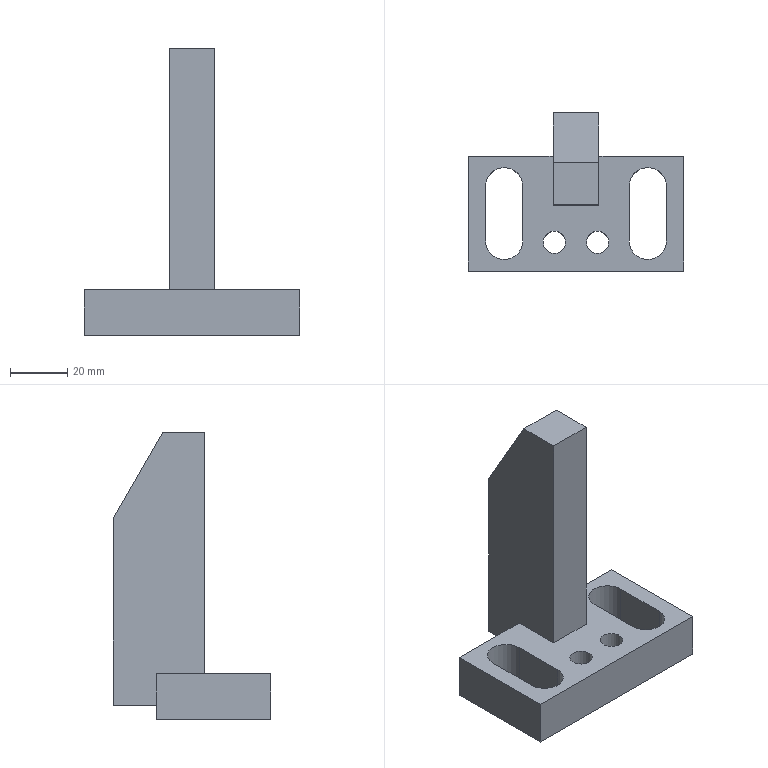Part | NX | features solid 2 | 1 solid | 23 faces | box 75 x 55 x 100 mm | volume 75811 mm3 | plane 17 | cylinder 6 | commonest cylinder face diameters 13 x4 7.8 x2
STEP:
#1=CARTESIAN_POINT('',(-292.,-815.,61.));
#2=VERTEX_POINT('',#1);
#3=CARTESIAN_POINT('',(-292.,-832.,61.));
#4=VERTEX_POINT('',#3);
#5=CARTESIAN_POINT('',(-292.,-835.,61.));
#6=DIRECTION('',(0.,-1.,0.));
#7=VECTOR('',#6,1000.);
#8=LINE('',#5,#7);
#9=EDGE_CURVE('',#2,#4,#8,.T.);
#10=ORIENTED_EDGE('',*,*,#9,.T.);
#11=CARTESIAN_POINT('',(-308.,-832.,61.));
#12=VERTEX_POINT('',#11);
#13=CARTESIAN_POINT('',(-300.,-832.,61.));
#14=DIRECTION('',(-1.,0.,0.));
#15=VECTOR('',#14,1000.);
#16=LINE('',#13,#15);
#17=EDGE_CURVE('',#4,#12,#16,.T.);
#18=ORIENTED_EDGE('',*,*,#17,.T.);
#19=CARTESIAN_POINT('',(-308.,-815.,61.));
#20=VERTEX_POINT('',#19);
#21=CARTESIAN_POINT('',(-308.,-835.,61.));
#22=DIRECTION('',(0.,1.,0.));
#23=VECTOR('',#22,1000.);
#24=LINE('',#21,#23);
#25=EDGE_CURVE('',#12,#20,#24,.T.);
#26=ORIENTED_EDGE('',*,*,#25,.T.);
#27=CARTESIAN_POINT('',(-337.5,-815.,61.));
#28=VERTEX_POINT('',#27);
#29=CARTESIAN_POINT('',(-300.,-815.,61.));
#30=DIRECTION('',(-1.,0.,0.));
#31=VECTOR('',#30,1000.);
#32=LINE('',#29,#31);
#33=EDGE_CURVE('',#20,#28,#32,.T.);
#34=ORIENTED_EDGE('',*,*,#33,.T.);
#35=CARTESIAN_POINT('',(-337.5,-855.,61.));
#36=VERTEX_POINT('',#35);
#37=CARTESIAN_POINT('',(-337.5,-835.,61.));
#38=DIRECTION('',(0.,-1.,0.));
#39=VECTOR('',#38,1000.);
#40=LINE('',#37,#39);
#41=EDGE_CURVE('',#28,#36,#40,.T.);
#42=ORIENTED_EDGE('',*,*,#41,.T.);
#43=CARTESIAN_POINT('',(-262.5,-855.,61.));
#44=VERTEX_POINT('',#43);
#45=CARTESIAN_POINT('',(-300.,-855.,61.));
#46=DIRECTION('',(1.,0.,0.));
#47=VECTOR('',#46,1000.);
#48=LINE('',#45,#47);
#49=EDGE_CURVE('',#36,#44,#48,.T.);
#50=ORIENTED_EDGE('',*,*,#49,.T.);
#51=CARTESIAN_POINT('',(-262.5,-815.,61.));
#52=VERTEX_POINT('',#51);
#53=CARTESIAN_POINT('',(-262.5,-835.,61.));
#54=DIRECTION('',(0.,1.,0.));
#55=VECTOR('',#54,1000.);
#56=LINE('',#53,#55);
#57=EDGE_CURVE('',#44,#52,#56,.T.);
#58=ORIENTED_EDGE('',*,*,#57,.T.);
#59=CARTESIAN_POINT('',(-300.,-815.,61.));
#60=DIRECTION('',(-1.,0.,0.));
#61=VECTOR('',#60,1000.);
#62=LINE('',#59,#61);
#63=EDGE_CURVE('',#52,#2,#62,.T.);
#64=ORIENTED_EDGE('',*,*,#63,.T.);
#65=EDGE_LOOP('',(#10,#18,#26,#34,#42,#50,#58,#64));
#66=FACE_BOUND('',#65,.T.);
#67=CARTESIAN_POINT('',(-318.5,-825.5,61.));
#68=VERTEX_POINT('',#67);
#69=CARTESIAN_POINT('',(-331.5,-825.5,61.));
#70=VERTEX_POINT('',#69);
#71=CARTESIAN_POINT('',(-325.,-825.5,61.));
#72=DIRECTION('',(0.,0.,1.));
#73=DIRECTION('',(0.,1.,0.));
#74=AXIS2_PLACEMENT_3D('',#71,#72,#73);
#75=CIRCLE('',#74,6.5);
#76=EDGE_CURVE('',#68,#70,#75,.T.);
#77=ORIENTED_EDGE('',*,*,#76,.F.);
#78=CARTESIAN_POINT('',(-318.5,-844.5,61.));
#79=VERTEX_POINT('',#78);
#80=CARTESIAN_POINT('',(-318.5,-835.,61.));
#81=DIRECTION('',(0.,1.,0.));
#82=VECTOR('',#81,1000.);
#83=LINE('',#80,#82);
#84=EDGE_CURVE('',#79,#68,#83,.T.);
#85=ORIENTED_EDGE('',*,*,#84,.F.);
#86=CARTESIAN_POINT('',(-331.5,-844.5,61.));
#87=VERTEX_POINT('',#86);
#88=CARTESIAN_POINT('',(-325.,-844.5,61.));
#89=DIRECTION('',(0.,0.,1.));
#90=DIRECTION('',(0.,1.,0.));
#91=AXIS2_PLACEMENT_3D('',#88,#89,#90);
#92=CIRCLE('',#91,6.5);
#93=EDGE_CURVE('',#87,#79,#92,.T.);
#94=ORIENTED_EDGE('',*,*,#93,.F.);
#95=CARTESIAN_POINT('',(-331.5,-835.,61.));
#96=DIRECTION('',(0.,-1.,0.));
#97=VECTOR('',#96,1000.);
#98=LINE('',#95,#97);
#99=EDGE_CURVE('',#70,#87,#98,.T.);
#100=ORIENTED_EDGE('',*,*,#99,.F.);
#101=EDGE_LOOP('',(#77,#85,#94,#100));
#102=FACE_BOUND('',#101,.T.);
#103=CARTESIAN_POINT('',(-268.5,-825.5,61.));
#104=VERTEX_POINT('',#103);
#105=CARTESIAN_POINT('',(-281.5,-825.5,61.));
#106=VERTEX_POINT('',#105);
#107=CARTESIAN_POINT('',(-275.,-825.5,61.));
#108=DIRECTION('',(0.,0.,1.));
#109=DIRECTION('',(0.,1.,0.));
#110=AXIS2_PLACEMENT_3D('',#107,#108,#109);
#111=CIRCLE('',#110,6.5);
#112=EDGE_CURVE('',#104,#106,#111,.T.);
#113=ORIENTED_EDGE('',*,*,#112,.F.);
#114=CARTESIAN_POINT('',(-268.5,-844.5,61.));
#115=VERTEX_POINT('',#114);
#116=CARTESIAN_POINT('',(-268.5,-835.,61.));
#117=DIRECTION('',(0.,1.,0.));
#118=VECTOR('',#117,1000.);
#119=LINE('',#116,#118);
#120=EDGE_CURVE('',#115,#104,#119,.T.);
#121=ORIENTED_EDGE('',*,*,#120,.F.);
#122=CARTESIAN_POINT('',(-281.5,-844.5,61.));
#123=VERTEX_POINT('',#122);
#124=CARTESIAN_POINT('',(-275.,-844.5,61.));
#125=DIRECTION('',(0.,0.,1.));
#126=DIRECTION('',(0.,1.,0.));
#127=AXIS2_PLACEMENT_3D('',#124,#125,#126);
#128=CIRCLE('',#127,6.5);
#129=EDGE_CURVE('',#123,#115,#128,.T.);
#130=ORIENTED_EDGE('',*,*,#129,.F.);
#131=CARTESIAN_POINT('',(-281.5,-835.,61.));
#132=DIRECTION('',(0.,-1.,0.));
#133=VECTOR('',#132,1000.);
#134=LINE('',#131,#133);
#135=EDGE_CURVE('',#106,#123,#134,.T.);
#136=ORIENTED_EDGE('',*,*,#135,.F.);
#137=EDGE_LOOP('',(#113,#121,#130,#136));
#138=FACE_BOUND('',#137,.T.);
#139=CARTESIAN_POINT('',(-307.5,-841.1,61.));
#140=VERTEX_POINT('',#139);
#141=CARTESIAN_POINT('',(-307.5,-845.,61.));
#142=DIRECTION('',(0.,0.,1.));
#143=DIRECTION('',(0.,1.,0.));
#144=AXIS2_PLACEMENT_3D('',#141,#142,#143);
#145=CIRCLE('',#144,3.9);
#146=EDGE_CURVE('',#140,#140,#145,.T.);
#147=ORIENTED_EDGE('',*,*,#146,.F.);
#148=EDGE_LOOP('',(#147));
#149=FACE_BOUND('',#148,.T.);
#150=CARTESIAN_POINT('',(-292.5,-841.1,61.));
#151=VERTEX_POINT('',#150);
#152=CARTESIAN_POINT('',(-292.5,-845.,61.));
#153=DIRECTION('',(0.,0.,1.));
#154=DIRECTION('',(0.,1.,0.));
#155=AXIS2_PLACEMENT_3D('',#152,#153,#154);
#156=CIRCLE('',#155,3.9);
#157=EDGE_CURVE('',#151,#151,#156,.T.);
#158=ORIENTED_EDGE('',*,*,#157,.F.);
#159=EDGE_LOOP('',(#158));
#160=FACE_BOUND('',#159,.T.);
#161=CARTESIAN_POINT('',(-300.,-835.,61.));
#162=DIRECTION('',(0.,0.,1.));
#163=DIRECTION('',(0.,-1.,0.));
#164=AXIS2_PLACEMENT_3D('',#161,#162,#163);
#165=PLANE('',#164);
#166=ADVANCED_FACE('',(#66,#102,#138,#149,#160),#165,.T.);
#167=CARTESIAN_POINT('',(-262.5,-855.,45.));
#168=VERTEX_POINT('',#167);
#169=CARTESIAN_POINT('',(-262.5,-855.,45.));
#170=DIRECTION('',(0.,0.,1.));
#171=VECTOR('',#170,1000.);
#172=LINE('',#169,#171);
#173=EDGE_CURVE('',#168,#44,#172,.T.);
#174=ORIENTED_EDGE('',*,*,#173,.F.);
#175=CARTESIAN_POINT('',(-262.5,-815.,45.));
#176=VERTEX_POINT('',#175);
#177=CARTESIAN_POINT('',(-262.5,-835.,45.));
#178=DIRECTION('',(0.,-1.,0.));
#179=VECTOR('',#178,1000.);
#180=LINE('',#177,#179);
#181=EDGE_CURVE('',#176,#168,#180,.T.);
#182=ORIENTED_EDGE('',*,*,#181,.F.);
#183=CARTESIAN_POINT('',(-262.5,-815.,45.));
#184=DIRECTION('',(0.,0.,1.));
#185=VECTOR('',#184,1000.);
#186=LINE('',#183,#185);
#187=EDGE_CURVE('',#176,#52,#186,.T.);
#188=ORIENTED_EDGE('',*,*,#187,.T.);
#189=ORIENTED_EDGE('',*,*,#57,.F.);
#190=EDGE_LOOP('',(#174,#182,#188,#189));
#191=FACE_BOUND('',#190,.T.);
#192=CARTESIAN_POINT('',(-262.5,-835.,45.));
#193=DIRECTION('',(1.,0.,0.));
#194=DIRECTION('',(0.,0.,-1.));
#195=AXIS2_PLACEMENT_3D('',#192,#193,#194);
#196=PLANE('',#195);
#197=ADVANCED_FACE('',(#191),#196,.T.);
#198=CARTESIAN_POINT('',(-292.,-815.,50.));
#199=VERTEX_POINT('',#198);
#200=CARTESIAN_POINT('',(-292.,-815.,45.));
#201=DIRECTION('',(0.,0.,1.));
#202=VECTOR('',#201,1000.);
#203=LINE('',#200,#202);
#204=EDGE_CURVE('',#199,#2,#203,.T.);
#205=ORIENTED_EDGE('',*,*,#204,.T.);
#206=ORIENTED_EDGE('',*,*,#63,.F.);
#207=ORIENTED_EDGE('',*,*,#187,.F.);
#208=CARTESIAN_POINT('',(-337.5,-815.,45.));
#209=VERTEX_POINT('',#208);
#210=CARTESIAN_POINT('',(-300.,-815.,45.));
#211=DIRECTION('',(1.,0.,0.));
#212=VECTOR('',#211,1000.);
#213=LINE('',#210,#212);
#214=EDGE_CURVE('',#209,#176,#213,.T.);
#215=ORIENTED_EDGE('',*,*,#214,.F.);
#216=CARTESIAN_POINT('',(-337.5,-815.,45.));
#217=DIRECTION('',(0.,0.,1.));
#218=VECTOR('',#217,1000.);
#219=LINE('',#216,#218);
#220=EDGE_CURVE('',#209,#28,#219,.T.);
#221=ORIENTED_EDGE('',*,*,#220,.T.);
#222=ORIENTED_EDGE('',*,*,#33,.F.);
#223=CARTESIAN_POINT('',(-308.,-815.,50.));
#224=VERTEX_POINT('',#223);
#225=CARTESIAN_POINT('',(-308.,-815.,45.));
#226=DIRECTION('',(0.,0.,-1.));
#227=VECTOR('',#226,1000.);
#228=LINE('',#225,#227);
#229=EDGE_CURVE('',#20,#224,#228,.T.);
#230=ORIENTED_EDGE('',*,*,#229,.T.);
#231=CARTESIAN_POINT('',(-300.,-815.,50.));
#232=DIRECTION('',(1.,0.,0.));
#233=VECTOR('',#232,1000.);
#234=LINE('',#231,#233);
#235=EDGE_CURVE('',#224,#199,#234,.T.);
#236=ORIENTED_EDGE('',*,*,#235,.T.);
#237=EDGE_LOOP('',(#205,#206,#207,#215,#221,#222,#230,#236));
#238=FACE_BOUND('',#237,.T.);
#239=CARTESIAN_POINT('',(-300.,-815.,45.));
#240=DIRECTION('',(0.,1.,0.));
#241=DIRECTION('',(0.,0.,1.));
#242=AXIS2_PLACEMENT_3D('',#239,#240,#241);
#243=PLANE('',#242);
#244=ADVANCED_FACE('',(#238),#243,.T.);
#245=ORIENTED_EDGE('',*,*,#220,.F.);
#246=CARTESIAN_POINT('',(-337.5,-855.,45.));
#247=VERTEX_POINT('',#246);
#248=CARTESIAN_POINT('',(-337.5,-835.,45.));
#249=DIRECTION('',(0.,1.,0.));
#250=VECTOR('',#249,1000.);
#251=LINE('',#248,#250);
#252=EDGE_CURVE('',#247,#209,#251,.T.);
#253=ORIENTED_EDGE('',*,*,#252,.F.);
#254=CARTESIAN_POINT('',(-337.5,-855.,45.));
#255=DIRECTION('',(0.,0.,1.));
#256=VECTOR('',#255,1000.);
#257=LINE('',#254,#256);
#258=EDGE_CURVE('',#247,#36,#257,.T.);
#259=ORIENTED_EDGE('',*,*,#258,.T.);
#260=ORIENTED_EDGE('',*,*,#41,.F.);
#261=EDGE_LOOP('',(#245,#253,#259,#260));
#262=FACE_BOUND('',#261,.T.);
#263=CARTESIAN_POINT('',(-337.5,-835.,45.));
#264=DIRECTION('',(-1.,0.,0.));
#265=DIRECTION('',(0.,0.,1.));
#266=AXIS2_PLACEMENT_3D('',#263,#264,#265);
#267=PLANE('',#266);
#268=ADVANCED_FACE('',(#262),#267,.T.);
#269=CARTESIAN_POINT('',(-331.5,-825.5,45.));
#270=VERTEX_POINT('',#269);
#271=CARTESIAN_POINT('',(-318.5,-825.5,45.));
#272=VERTEX_POINT('',#271);
#273=CARTESIAN_POINT('',(-325.,-825.5,45.));
#274=DIRECTION('',(0.,0.,-1.));
#275=DIRECTION('',(0.,-1.,0.));
#276=AXIS2_PLACEMENT_3D('',#273,#274,#275);
#277=CIRCLE('',#276,6.5);
#278=EDGE_CURVE('',#270,#272,#277,.T.);
#279=ORIENTED_EDGE('',*,*,#278,.F.);
#280=CARTESIAN_POINT('',(-331.5,-844.5,45.));
#281=VERTEX_POINT('',#280);
#282=CARTESIAN_POINT('',(-331.5,-835.,45.));
#283=DIRECTION('',(0.,1.,0.));
#284=VECTOR('',#283,1000.);
#285=LINE('',#282,#284);
#286=EDGE_CURVE('',#281,#270,#285,.T.);
#287=ORIENTED_EDGE('',*,*,#286,.F.);
#288=CARTESIAN_POINT('',(-318.5,-844.5,45.));
#289=VERTEX_POINT('',#288);
#290=CARTESIAN_POINT('',(-325.,-844.5,45.));
#291=DIRECTION('',(0.,0.,-1.));
#292=DIRECTION('',(0.,-1.,0.));
#293=AXIS2_PLACEMENT_3D('',#290,#291,#292);
#294=CIRCLE('',#293,6.5);
#295=EDGE_CURVE('',#289,#281,#294,.T.);
#296=ORIENTED_EDGE('',*,*,#295,.F.);
#297=CARTESIAN_POINT('',(-318.5,-835.,45.));
#298=DIRECTION('',(0.,-1.,0.));
#299=VECTOR('',#298,1000.);
#300=LINE('',#297,#299);
#301=EDGE_CURVE('',#272,#289,#300,.T.);
#302=ORIENTED_EDGE('',*,*,#301,.F.);
#303=EDGE_LOOP('',(#279,#287,#296,#302));
#304=FACE_BOUND('',#303,.T.);
#305=CARTESIAN_POINT('',(-281.5,-825.5,45.));
#306=VERTEX_POINT('',#305);
#307=CARTESIAN_POINT('',(-268.5,-825.5,45.));
#308=VERTEX_POINT('',#307);
#309=CARTESIAN_POINT('',(-275.,-825.5,45.));
#310=DIRECTION('',(0.,0.,-1.));
#311=DIRECTION('',(0.,-1.,0.));
#312=AXIS2_PLACEMENT_3D('',#309,#310,#311);
#313=CIRCLE('',#312,6.5);
#314=EDGE_CURVE('',#306,#308,#313,.T.);
#315=ORIENTED_EDGE('',*,*,#314,.F.);
#316=CARTESIAN_POINT('',(-281.5,-844.5,45.));
#317=VERTEX_POINT('',#316);
#318=CARTESIAN_POINT('',(-281.5,-835.,45.));
#319=DIRECTION('',(0.,1.,0.));
#320=VECTOR('',#319,1000.);
#321=LINE('',#318,#320);
#322=EDGE_CURVE('',#317,#306,#321,.T.);
#323=ORIENTED_EDGE('',*,*,#322,.F.);
#324=CARTESIAN_POINT('',(-268.5,-844.5,45.));
#325=VERTEX_POINT('',#324);
#326=CARTESIAN_POINT('',(-275.,-844.5,45.));
#327=DIRECTION('',(0.,0.,-1.));
#328=DIRECTION('',(0.,-1.,0.));
#329=AXIS2_PLACEMENT_3D('',#326,#327,#328);
#330=CIRCLE('',#329,6.5);
#331=EDGE_CURVE('',#325,#317,#330,.T.);
#332=ORIENTED_EDGE('',*,*,#331,.F.);
#333=CARTESIAN_POINT('',(-268.5,-835.,45.));
#334=DIRECTION('',(0.,-1.,0.));
#335=VECTOR('',#334,1000.);
#336=LINE('',#333,#335);
#337=EDGE_CURVE('',#308,#325,#336,.T.);
#338=ORIENTED_EDGE('',*,*,#337,.F.);
#339=EDGE_LOOP('',(#315,#323,#332,#338));
#340=FACE_BOUND('',#339,.T.);
#341=CARTESIAN_POINT('',(-307.5,-848.9,45.));
#342=VERTEX_POINT('',#341);
#343=CARTESIAN_POINT('',(-307.5,-845.,45.));
#344=DIRECTION('',(0.,0.,-1.));
#345=DIRECTION('',(0.,-1.,0.));
#346=AXIS2_PLACEMENT_3D('',#343,#344,#345);
#347=CIRCLE('',#346,3.9);
#348=EDGE_CURVE('',#342,#342,#347,.T.);
#349=ORIENTED_EDGE('',*,*,#348,.F.);
#350=EDGE_LOOP('',(#349));
#351=FACE_BOUND('',#350,.T.);
#352=CARTESIAN_POINT('',(-292.5,-848.9,45.));
#353=VERTEX_POINT('',#352);
#354=CARTESIAN_POINT('',(-292.5,-845.,45.));
#355=DIRECTION('',(0.,0.,-1.));
#356=DIRECTION('',(0.,-1.,0.));
#357=AXIS2_PLACEMENT_3D('',#354,#355,#356);
#358=CIRCLE('',#357,3.9);
#359=EDGE_CURVE('',#353,#353,#358,.T.);
#360=ORIENTED_EDGE('',*,*,#359,.F.);
#361=EDGE_LOOP('',(#360));
#362=FACE_BOUND('',#361,.T.);
#363=CARTESIAN_POINT('',(-300.,-855.,45.));
#364=DIRECTION('',(-1.,0.,0.));
#365=VECTOR('',#364,1000.);
#366=LINE('',#363,#365);
#367=EDGE_CURVE('',#168,#247,#366,.T.);
#368=ORIENTED_EDGE('',*,*,#367,.T.);
#369=ORIENTED_EDGE('',*,*,#252,.T.);
#370=ORIENTED_EDGE('',*,*,#214,.T.);
#371=ORIENTED_EDGE('',*,*,#181,.T.);
#372=EDGE_LOOP('',(#368,#369,#370,#371));
#373=FACE_BOUND('',#372,.T.);
#374=CARTESIAN_POINT('',(-300.,-835.,45.));
#375=DIRECTION('',(0.,0.,-1.));
#376=DIRECTION('',(0.,1.,0.));
#377=AXIS2_PLACEMENT_3D('',#374,#375,#376);
#378=PLANE('',#377);
#379=ADVANCED_FACE('',(#304,#340,#351,#362,#373),#378,.T.);
#380=ORIENTED_EDGE('',*,*,#367,.F.);
#381=ORIENTED_EDGE('',*,*,#173,.T.);
#382=ORIENTED_EDGE('',*,*,#49,.F.);
#383=ORIENTED_EDGE('',*,*,#258,.F.);
#384=EDGE_LOOP('',(#380,#381,#382,#383));
#385=FACE_BOUND('',#384,.T.);
#386=CARTESIAN_POINT('',(-300.,-855.,45.));
#387=DIRECTION('',(0.,-1.,0.));
#388=DIRECTION('',(0.,0.,-1.));
#389=AXIS2_PLACEMENT_3D('',#386,#387,#388);
#390=PLANE('',#389);
#391=ADVANCED_FACE('',(#385),#390,.T.);
#392=ORIENTED_EDGE('',*,*,#157,.T.);
#393=EDGE_LOOP('',(#392));
#394=FACE_BOUND('',#393,.T.);
#395=ORIENTED_EDGE('',*,*,#359,.T.);
#396=EDGE_LOOP('',(#395));
#397=FACE_BOUND('',#396,.T.);
#398=CARTESIAN_POINT('',(-292.5,-845.,45.));
#399=DIRECTION('',(0.,0.,1.));
#400=DIRECTION('',(0.,-1.,0.));
#401=AXIS2_PLACEMENT_3D('',#398,#399,#400);
#402=CYLINDRICAL_SURFACE('',#401,3.9);
#403=ADVANCED_FACE('',(#394,#397),#402,.F.);
#404=ORIENTED_EDGE('',*,*,#146,.T.);
#405=EDGE_LOOP('',(#404));
#406=FACE_BOUND('',#405,.T.);
#407=ORIENTED_EDGE('',*,*,#348,.T.);
#408=EDGE_LOOP('',(#407));
#409=FACE_BOUND('',#408,.T.);
#410=CARTESIAN_POINT('',(-307.5,-845.,45.));
#411=DIRECTION('',(0.,0.,1.));
#412=DIRECTION('',(0.,-1.,0.));
#413=AXIS2_PLACEMENT_3D('',#410,#411,#412);
#414=CYLINDRICAL_SURFACE('',#413,3.9);
#415=ADVANCED_FACE('',(#406,#409),#414,.F.);
#416=CARTESIAN_POINT('',(-268.5,-844.5,45.));
#417=DIRECTION('',(0.,0.,1.));
#418=VECTOR('',#417,1000.);
#419=LINE('',#416,#418);
#420=EDGE_CURVE('',#325,#115,#419,.T.);
#421=ORIENTED_EDGE('',*,*,#420,.T.);
#422=ORIENTED_EDGE('',*,*,#120,.T.);
#423=CARTESIAN_POINT('',(-268.5,-825.5,45.));
#424=DIRECTION('',(0.,0.,1.));
#425=VECTOR('',#424,1000.);
#426=LINE('',#423,#425);
#427=EDGE_CURVE('',#308,#104,#426,.T.);
#428=ORIENTED_EDGE('',*,*,#427,.F.);
#429=ORIENTED_EDGE('',*,*,#337,.T.);
#430=EDGE_LOOP('',(#421,#422,#428,#429));
#431=FACE_BOUND('',#430,.T.);
#432=CARTESIAN_POINT('',(-268.5,-835.,45.));
#433=DIRECTION('',(1.,0.,0.));
#434=DIRECTION('',(0.,0.,-1.));
#435=AXIS2_PLACEMENT_3D('',#432,#433,#434);
#436=PLANE('',#435);
#437=ADVANCED_FACE('',(#431),#436,.F.);
#438=CARTESIAN_POINT('',(-281.5,-825.5,45.));
#439=DIRECTION('',(0.,0.,1.));
#440=VECTOR('',#439,1000.);
#441=LINE('',#438,#440);
#442=EDGE_CURVE('',#306,#106,#441,.T.);
#443=ORIENTED_EDGE('',*,*,#442,.T.);
#444=ORIENTED_EDGE('',*,*,#135,.T.);
#445=CARTESIAN_POINT('',(-281.5,-844.5,45.));
#446=DIRECTION('',(0.,0.,1.));
#447=VECTOR('',#446,1000.);
#448=LINE('',#445,#447);
#449=EDGE_CURVE('',#317,#123,#448,.T.);
#450=ORIENTED_EDGE('',*,*,#449,.F.);
#451=ORIENTED_EDGE('',*,*,#322,.T.);
#452=EDGE_LOOP('',(#443,#444,#450,#451));
#453=FACE_BOUND('',#452,.T.);
#454=CARTESIAN_POINT('',(-281.5,-835.,45.));
#455=DIRECTION('',(-1.,0.,0.));
#456=DIRECTION('',(0.,0.,1.));
#457=AXIS2_PLACEMENT_3D('',#454,#455,#456);
#458=PLANE('',#457);
#459=ADVANCED_FACE('',(#453),#458,.F.);
#460=ORIENTED_EDGE('',*,*,#314,.T.);
#461=ORIENTED_EDGE('',*,*,#427,.T.);
#462=ORIENTED_EDGE('',*,*,#112,.T.);
#463=ORIENTED_EDGE('',*,*,#442,.F.);
#464=EDGE_LOOP('',(#460,#461,#462,#463));
#465=FACE_BOUND('',#464,.T.);
#466=CARTESIAN_POINT('',(-275.,-825.5,45.));
#467=DIRECTION('',(0.,0.,1.));
#468=DIRECTION('',(0.,-1.,0.));
#469=AXIS2_PLACEMENT_3D('',#466,#467,#468);
#470=CYLINDRICAL_SURFACE('',#469,6.5);
#471=ADVANCED_FACE('',(#465),#470,.F.);
#472=ORIENTED_EDGE('',*,*,#331,.T.);
#473=ORIENTED_EDGE('',*,*,#449,.T.);
#474=ORIENTED_EDGE('',*,*,#129,.T.);
#475=ORIENTED_EDGE('',*,*,#420,.F.);
#476=EDGE_LOOP('',(#472,#473,#474,#475));
#477=FACE_BOUND('',#476,.T.);
#478=CARTESIAN_POINT('',(-275.,-844.5,45.));
#479=DIRECTION('',(0.,0.,1.));
#480=DIRECTION('',(0.,-1.,0.));
#481=AXIS2_PLACEMENT_3D('',#478,#479,#480);
#482=CYLINDRICAL_SURFACE('',#481,6.5);
#483=ADVANCED_FACE('',(#477),#482,.F.);
#484=CARTESIAN_POINT('',(-318.5,-844.5,45.));
#485=DIRECTION('',(0.,0.,1.));
#486=VECTOR('',#485,1000.);
#487=LINE('',#484,#486);
#488=EDGE_CURVE('',#289,#79,#487,.T.);
#489=ORIENTED_EDGE('',*,*,#488,.T.);
#490=ORIENTED_EDGE('',*,*,#84,.T.);
#491=CARTESIAN_POINT('',(-318.5,-825.5,45.));
#492=DIRECTION('',(0.,0.,1.));
#493=VECTOR('',#492,1000.);
#494=LINE('',#491,#493);
#495=EDGE_CURVE('',#272,#68,#494,.T.);
#496=ORIENTED_EDGE('',*,*,#495,.F.);
#497=ORIENTED_EDGE('',*,*,#301,.T.);
#498=EDGE_LOOP('',(#489,#490,#496,#497));
#499=FACE_BOUND('',#498,.T.);
#500=CARTESIAN_POINT('',(-318.5,-835.,45.));
#501=DIRECTION('',(1.,0.,0.));
#502=DIRECTION('',(0.,0.,-1.));
#503=AXIS2_PLACEMENT_3D('',#500,#501,#502);
#504=PLANE('',#503);
#505=ADVANCED_FACE('',(#499),#504,.F.);
#506=CARTESIAN_POINT('',(-331.5,-825.5,45.));
#507=DIRECTION('',(0.,0.,1.));
#508=VECTOR('',#507,1000.);
#509=LINE('',#506,#508);
#510=EDGE_CURVE('',#270,#70,#509,.T.);
#511=ORIENTED_EDGE('',*,*,#510,.T.);
#512=ORIENTED_EDGE('',*,*,#99,.T.);
#513=CARTESIAN_POINT('',(-331.5,-844.5,45.));
#514=DIRECTION('',(0.,0.,1.));
#515=VECTOR('',#514,1000.);
#516=LINE('',#513,#515);
#517=EDGE_CURVE('',#281,#87,#516,.T.);
#518=ORIENTED_EDGE('',*,*,#517,.F.);
#519=ORIENTED_EDGE('',*,*,#286,.T.);
#520=EDGE_LOOP('',(#511,#512,#518,#519));
#521=FACE_BOUND('',#520,.T.);
#522=CARTESIAN_POINT('',(-331.5,-835.,45.));
#523=DIRECTION('',(-1.,0.,0.));
#524=DIRECTION('',(0.,0.,1.));
#525=AXIS2_PLACEMENT_3D('',#522,#523,#524);
#526=PLANE('',#525);
#527=ADVANCED_FACE('',(#521),#526,.F.);
#528=ORIENTED_EDGE('',*,*,#278,.T.);
#529=ORIENTED_EDGE('',*,*,#495,.T.);
#530=ORIENTED_EDGE('',*,*,#76,.T.);
#531=ORIENTED_EDGE('',*,*,#510,.F.);
#532=EDGE_LOOP('',(#528,#529,#530,#531));
#533=FACE_BOUND('',#532,.T.);
#534=CARTESIAN_POINT('',(-325.,-825.5,45.));
#535=DIRECTION('',(0.,0.,1.));
#536=DIRECTION('',(0.,-1.,0.));
#537=AXIS2_PLACEMENT_3D('',#534,#535,#536);
#538=CYLINDRICAL_SURFACE('',#537,6.5);
#539=ADVANCED_FACE('',(#533),#538,.F.);
#540=ORIENTED_EDGE('',*,*,#295,.T.);
#541=ORIENTED_EDGE('',*,*,#517,.T.);
#542=ORIENTED_EDGE('',*,*,#93,.T.);
#543=ORIENTED_EDGE('',*,*,#488,.F.);
#544=EDGE_LOOP('',(#540,#541,#542,#543));
#545=FACE_BOUND('',#544,.T.);
#546=CARTESIAN_POINT('',(-325.,-844.5,45.));
#547=DIRECTION('',(0.,0.,1.));
#548=DIRECTION('',(0.,-1.,0.));
#549=AXIS2_PLACEMENT_3D('',#546,#547,#548);
#550=CYLINDRICAL_SURFACE('',#549,6.5);
#551=ADVANCED_FACE('',(#545),#550,.F.);
#552=CARTESIAN_POINT('',(-292.,-817.321,145.));
#553=VERTEX_POINT('',#552);
#554=CARTESIAN_POINT('',(-308.,-817.321,145.));
#555=VERTEX_POINT('',#554);
#556=CARTESIAN_POINT('',(-300.,-817.321,145.));
#557=DIRECTION('',(-1.,0.,0.));
#558=VECTOR('',#557,1000.);
#559=LINE('',#556,#558);
#560=EDGE_CURVE('',#553,#555,#559,.T.);
#561=ORIENTED_EDGE('',*,*,#560,.T.);
#562=CARTESIAN_POINT('',(-308.,-832.,145.));
#563=VERTEX_POINT('',#562);
#564=CARTESIAN_POINT('',(-308.,-816.,145.));
#565=DIRECTION('',(0.,-1.,0.));
#566=VECTOR('',#565,1000.);
#567=LINE('',#564,#566);
#568=EDGE_CURVE('',#555,#563,#567,.T.);
#569=ORIENTED_EDGE('',*,*,#568,.T.);
#570=CARTESIAN_POINT('',(-292.,-832.,145.));
#571=VERTEX_POINT('',#570);
#572=CARTESIAN_POINT('',(-300.,-832.,145.));
#573=DIRECTION('',(1.,0.,0.));
#574=VECTOR('',#573,1000.);
#575=LINE('',#572,#574);
#576=EDGE_CURVE('',#563,#571,#575,.T.);
#577=ORIENTED_EDGE('',*,*,#576,.T.);
#578=CARTESIAN_POINT('',(-292.,-816.,145.));
#579=DIRECTION('',(0.,1.,0.));
#580=VECTOR('',#579,1000.);
#581=LINE('',#578,#580);
#582=EDGE_CURVE('',#571,#553,#581,.T.);
#583=ORIENTED_EDGE('',*,*,#582,.T.);
#584=EDGE_LOOP('',(#561,#569,#577,#583));
#585=FACE_BOUND('',#584,.T.);
#586=CARTESIAN_POINT('',(-300.,-816.,145.));
#587=DIRECTION('',(0.,0.,1.));
#588=DIRECTION('',(0.,-1.,0.));
#589=AXIS2_PLACEMENT_3D('',#586,#587,#588);
#590=PLANE('',#589);
#591=ADVANCED_FACE('',(#585),#590,.T.);
#592=ORIENTED_EDGE('',*,*,#204,.F.);
#593=CARTESIAN_POINT('',(-292.,-800.,50.));
#594=VERTEX_POINT('',#593);
#595=CARTESIAN_POINT('',(-292.,-816.,50.));
#596=DIRECTION('',(0.,-1.,0.));
#597=VECTOR('',#596,1000.);
#598=LINE('',#595,#597);
#599=EDGE_CURVE('',#594,#199,#598,.T.);
#600=ORIENTED_EDGE('',*,*,#599,.F.);
#601=CARTESIAN_POINT('',(-292.,-800.,115.));
#602=VERTEX_POINT('',#601);
#603=CARTESIAN_POINT('',(-292.,-800.,50.));
#604=DIRECTION('',(0.,0.,1.));
#605=VECTOR('',#604,1000.);
#606=LINE('',#603,#605);
#607=EDGE_CURVE('',#594,#602,#606,.T.);
#608=ORIENTED_EDGE('',*,*,#607,.T.);
#609=CARTESIAN_POINT('',(-292.,-800.,115.));
#610=DIRECTION('',(0.,-0.5,0.866));
#611=VECTOR('',#610,1000.);
#612=LINE('',#609,#611);
#613=EDGE_CURVE('',#602,#553,#612,.T.);
#614=ORIENTED_EDGE('',*,*,#613,.T.);
#615=ORIENTED_EDGE('',*,*,#582,.F.);
#616=CARTESIAN_POINT('',(-292.,-832.,50.));
#617=DIRECTION('',(0.,0.,1.));
#618=VECTOR('',#617,1000.);
#619=LINE('',#616,#618);
#620=EDGE_CURVE('',#4,#571,#619,.T.);
#621=ORIENTED_EDGE('',*,*,#620,.F.);
#622=ORIENTED_EDGE('',*,*,#9,.F.);
#623=EDGE_LOOP('',(#592,#600,#608,#614,#615,#621,#622));
#624=FACE_BOUND('',#623,.T.);
#625=CARTESIAN_POINT('',(-292.,-816.,50.));
#626=DIRECTION('',(1.,0.,0.));
#627=DIRECTION('',(0.,0.,-1.));
#628=AXIS2_PLACEMENT_3D('',#625,#626,#627);
#629=PLANE('',#628);
#630=ADVANCED_FACE('',(#624),#629,.T.);
#631=CARTESIAN_POINT('',(-308.,-800.,115.));
#632=VERTEX_POINT('',#631);
#633=CARTESIAN_POINT('',(-300.,-800.,115.));
#634=DIRECTION('',(-1.,0.,0.));
#635=VECTOR('',#634,1000.);
#636=LINE('',#633,#635);
#637=EDGE_CURVE('',#602,#632,#636,.T.);
#638=ORIENTED_EDGE('',*,*,#637,.F.);
#639=ORIENTED_EDGE('',*,*,#607,.F.);
#640=CARTESIAN_POINT('',(-308.,-800.,50.));
#641=VERTEX_POINT('',#640);
#642=CARTESIAN_POINT('',(-300.,-800.,50.));
#643=DIRECTION('',(1.,0.,0.));
#644=VECTOR('',#643,1000.);
#645=LINE('',#642,#644);
#646=EDGE_CURVE('',#641,#594,#645,.T.);
#647=ORIENTED_EDGE('',*,*,#646,.F.);
#648=CARTESIAN_POINT('',(-308.,-800.,50.));
#649=DIRECTION('',(0.,0.,1.));
#650=VECTOR('',#649,1000.);
#651=LINE('',#648,#650);
#652=EDGE_CURVE('',#641,#632,#651,.T.);
#653=ORIENTED_EDGE('',*,*,#652,.T.);
#654=EDGE_LOOP('',(#638,#639,#647,#653));
#655=FACE_BOUND('',#654,.T.);
#656=CARTESIAN_POINT('',(-300.,-800.,50.));
#657=DIRECTION('',(0.,1.,0.));
#658=DIRECTION('',(0.,0.,1.));
#659=AXIS2_PLACEMENT_3D('',#656,#657,#658);
#660=PLANE('',#659);
#661=ADVANCED_FACE('',(#655),#660,.T.);
#662=CARTESIAN_POINT('',(-308.,-832.,50.));
#663=DIRECTION('',(0.,0.,1.));
#664=VECTOR('',#663,1000.);
#665=LINE('',#662,#664);
#666=EDGE_CURVE('',#12,#563,#665,.T.);
#667=ORIENTED_EDGE('',*,*,#666,.T.);
#668=ORIENTED_EDGE('',*,*,#568,.F.);
#669=CARTESIAN_POINT('',(-308.,-800.,115.));
#670=DIRECTION('',(0.,-0.5,0.866));
#671=VECTOR('',#670,1000.);
#672=LINE('',#669,#671);
#673=EDGE_CURVE('',#632,#555,#672,.T.);
#674=ORIENTED_EDGE('',*,*,#673,.F.);
#675=ORIENTED_EDGE('',*,*,#652,.F.);
#676=CARTESIAN_POINT('',(-308.,-816.,50.));
#677=DIRECTION('',(0.,1.,0.));
#678=VECTOR('',#677,1000.);
#679=LINE('',#676,#678);
#680=EDGE_CURVE('',#224,#641,#679,.T.);
#681=ORIENTED_EDGE('',*,*,#680,.F.);
#682=ORIENTED_EDGE('',*,*,#229,.F.);
#683=ORIENTED_EDGE('',*,*,#25,.F.);
#684=EDGE_LOOP('',(#667,#668,#674,#675,#681,#682,#683));
#685=FACE_BOUND('',#684,.T.);
#686=CARTESIAN_POINT('',(-308.,-816.,50.));
#687=DIRECTION('',(-1.,0.,0.));
#688=DIRECTION('',(0.,0.,1.));
#689=AXIS2_PLACEMENT_3D('',#686,#687,#688);
#690=PLANE('',#689);
#691=ADVANCED_FACE('',(#685),#690,.T.);
#692=ORIENTED_EDGE('',*,*,#680,.T.);
#693=ORIENTED_EDGE('',*,*,#646,.T.);
#694=ORIENTED_EDGE('',*,*,#599,.T.);
#695=ORIENTED_EDGE('',*,*,#235,.F.);
#696=EDGE_LOOP('',(#692,#693,#694,#695));
#697=FACE_BOUND('',#696,.T.);
#698=CARTESIAN_POINT('',(-300.,-816.,50.));
#699=DIRECTION('',(0.,0.,-1.));
#700=DIRECTION('',(0.,1.,0.));
#701=AXIS2_PLACEMENT_3D('',#698,#699,#700);
#702=PLANE('',#701);
#703=ADVANCED_FACE('',(#697),#702,.T.);
#704=ORIENTED_EDGE('',*,*,#620,.T.);
#705=ORIENTED_EDGE('',*,*,#576,.F.);
#706=ORIENTED_EDGE('',*,*,#666,.F.);
#707=ORIENTED_EDGE('',*,*,#17,.F.);
#708=EDGE_LOOP('',(#704,#705,#706,#707));
#709=FACE_BOUND('',#708,.T.);
#710=CARTESIAN_POINT('',(-300.,-832.,50.));
#711=DIRECTION('',(0.,-1.,0.));
#712=DIRECTION('',(0.,0.,-1.));
#713=AXIS2_PLACEMENT_3D('',#710,#711,#712);
#714=PLANE('',#713);
#715=ADVANCED_FACE('',(#709),#714,.T.);
#716=ORIENTED_EDGE('',*,*,#560,.F.);
#717=ORIENTED_EDGE('',*,*,#613,.F.);
#718=ORIENTED_EDGE('',*,*,#637,.T.);
#719=ORIENTED_EDGE('',*,*,#673,.T.);
#720=EDGE_LOOP('',(#716,#717,#718,#719));
#721=FACE_BOUND('',#720,.T.);
#722=CARTESIAN_POINT('',(-300.,-800.,115.));
#723=DIRECTION('',(0.,-0.866,-0.5));
#724=DIRECTION('',(0.,0.5,-0.866));
#725=AXIS2_PLACEMENT_3D('',#722,#723,#724);
#726=PLANE('',#725);
#727=ADVANCED_FACE('',(#721),#726,.F.);
#728=CLOSED_SHELL('',(#166,#197,#244,#268,#379,#391,#403,#415,#437,#459,#471,#483,#505,#527,#539,#551,#591,#630,#661,#691,#703,#715,#727));
#729=MANIFOLD_SOLID_BREP('',#728);
#730=(LENGTH_UNIT()NAMED_UNIT(*)SI_UNIT(.MILLI.,.METRE.));
#731=UNCERTAINTY_MEASURE_WITH_UNIT(LENGTH_MEASURE(0.00001),#730,'','');
#732=(NAMED_UNIT(*)PLANE_ANGLE_UNIT()SI_UNIT($,.RADIAN.));
#733=(NAMED_UNIT(*)SI_UNIT($,.STERADIAN.)SOLID_ANGLE_UNIT());
#734=(GEOMETRIC_REPRESENTATION_CONTEXT(3)GLOBAL_UNCERTAINTY_ASSIGNED_CONTEXT((#731))GLOBAL_UNIT_ASSIGNED_CONTEXT((#730,#732,#733))REPRESENTATION_CONTEXT('',''));
#735=ADVANCED_BREP_SHAPE_REPRESENTATION('',(#729),#734);